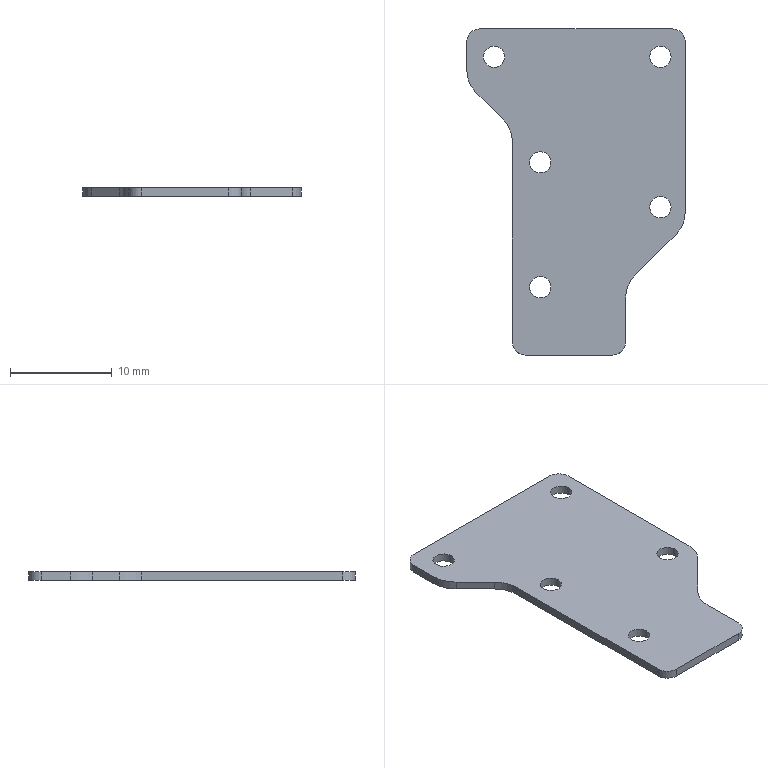Part | STEP file | Driver amplifier PA1PCB | 1 solid | 23 faces | box 21.48 x 32.08 x 0.832 mm | volume 418.678 mm3 | cylinder 13 | plane 10 | commonest cylinder face diameters 2.1 x5 2.54 x4 6.132 x4